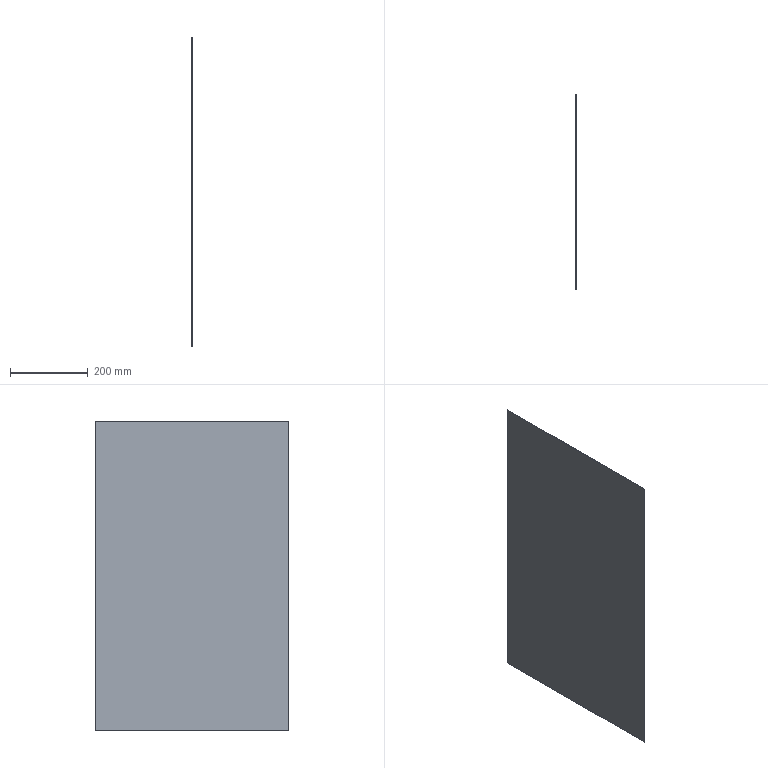Part | SolidWorks | features FlatPattern 1, SMBaseFlange 1, SheetMetal 1 | 1 solid | 6 faces | box 1.2 x 498.8 x 797.6 mm | volume 477411 mm3 | plane 6
STEP:
#1=CARTESIAN_POINT('',(165.125,151.045,-398.8));
#2=VERTEX_POINT('',#1);
#3=CARTESIAN_POINT('',(165.125,649.845,-398.8));
#4=VERTEX_POINT('',#3);
#5=CARTESIAN_POINT('',(165.125,151.045,-398.8));
#6=DIRECTION('',(0.,1.,0.));
#7=VECTOR('',#6,1000.);
#8=LINE('',#5,#7);
#9=EDGE_CURVE('',#2,#4,#8,.T.);
#10=ORIENTED_EDGE('',*,*,#9,.T.);
#11=CARTESIAN_POINT('',(165.125,649.845,398.8));
#12=VERTEX_POINT('',#11);
#13=CARTESIAN_POINT('',(165.125,649.845,398.8));
#14=DIRECTION('',(0.,0.,-1.));
#15=VECTOR('',#14,1000.);
#16=LINE('',#13,#15);
#17=EDGE_CURVE('',#12,#4,#16,.T.);
#18=ORIENTED_EDGE('',*,*,#17,.F.);
#19=CARTESIAN_POINT('',(165.125,151.045,398.8));
#20=VERTEX_POINT('',#19);
#21=CARTESIAN_POINT('',(165.125,151.045,398.8));
#22=DIRECTION('',(0.,1.,0.));
#23=VECTOR('',#22,1000.);
#24=LINE('',#21,#23);
#25=EDGE_CURVE('',#20,#12,#24,.T.);
#26=ORIENTED_EDGE('',*,*,#25,.F.);
#27=CARTESIAN_POINT('',(165.125,151.045,398.8));
#28=DIRECTION('',(0.,0.,-1.));
#29=VECTOR('',#28,1000.);
#30=LINE('',#27,#29);
#31=EDGE_CURVE('',#20,#2,#30,.T.);
#32=ORIENTED_EDGE('',*,*,#31,.T.);
#33=EDGE_LOOP('',(#10,#18,#26,#32));
#34=FACE_OUTER_BOUND('',#33,.T.);
#35=CARTESIAN_POINT('',(165.125,151.045,398.8));
#36=DIRECTION('',(-1.,0.,0.));
#37=DIRECTION('',(0.,0.,1.));
#38=AXIS2_PLACEMENT_3D('',#35,#36,#37);
#39=PLANE('',#38);
#40=ADVANCED_FACE('',(#34),#39,.F.);
#41=CARTESIAN_POINT('',(163.925,649.845,-398.8));
#42=VERTEX_POINT('',#41);
#43=CARTESIAN_POINT('',(163.925,649.845,-398.8));
#44=DIRECTION('',(1.,0.,0.));
#45=VECTOR('',#44,1000.);
#46=LINE('',#43,#45);
#47=EDGE_CURVE('',#42,#4,#46,.T.);
#48=ORIENTED_EDGE('',*,*,#47,.F.);
#49=CARTESIAN_POINT('',(163.925,649.845,398.8));
#50=VERTEX_POINT('',#49);
#51=CARTESIAN_POINT('',(163.925,649.845,398.8));
#52=DIRECTION('',(0.,0.,-1.));
#53=VECTOR('',#52,1000.);
#54=LINE('',#51,#53);
#55=EDGE_CURVE('',#50,#42,#54,.T.);
#56=ORIENTED_EDGE('',*,*,#55,.F.);
#57=CARTESIAN_POINT('',(163.925,649.845,398.8));
#58=DIRECTION('',(1.,0.,0.));
#59=VECTOR('',#58,1000.);
#60=LINE('',#57,#59);
#61=EDGE_CURVE('',#50,#12,#60,.T.);
#62=ORIENTED_EDGE('',*,*,#61,.T.);
#63=ORIENTED_EDGE('',*,*,#17,.T.);
#64=EDGE_LOOP('',(#48,#56,#62,#63));
#65=FACE_OUTER_BOUND('',#64,.T.);
#66=CARTESIAN_POINT('',(163.925,649.845,398.8));
#67=DIRECTION('',(0.,1.,0.));
#68=DIRECTION('',(0.,0.,1.));
#69=AXIS2_PLACEMENT_3D('',#66,#67,#68);
#70=PLANE('',#69);
#71=ADVANCED_FACE('',(#65),#70,.T.);
#72=CARTESIAN_POINT('',(163.925,151.045,-398.8));
#73=VERTEX_POINT('',#72);
#74=CARTESIAN_POINT('',(163.925,151.045,-398.8));
#75=DIRECTION('',(0.,1.,0.));
#76=VECTOR('',#75,1000.);
#77=LINE('',#74,#76);
#78=EDGE_CURVE('',#73,#42,#77,.T.);
#79=ORIENTED_EDGE('',*,*,#78,.F.);
#80=CARTESIAN_POINT('',(163.925,151.045,398.8));
#81=VERTEX_POINT('',#80);
#82=CARTESIAN_POINT('',(163.925,151.045,398.8));
#83=DIRECTION('',(0.,0.,-1.));
#84=VECTOR('',#83,1000.);
#85=LINE('',#82,#84);
#86=EDGE_CURVE('',#81,#73,#85,.T.);
#87=ORIENTED_EDGE('',*,*,#86,.F.);
#88=CARTESIAN_POINT('',(163.925,151.045,398.8));
#89=DIRECTION('',(0.,1.,0.));
#90=VECTOR('',#89,1000.);
#91=LINE('',#88,#90);
#92=EDGE_CURVE('',#81,#50,#91,.T.);
#93=ORIENTED_EDGE('',*,*,#92,.T.);
#94=ORIENTED_EDGE('',*,*,#55,.T.);
#95=EDGE_LOOP('',(#79,#87,#93,#94));
#96=FACE_OUTER_BOUND('',#95,.T.);
#97=CARTESIAN_POINT('',(163.925,151.045,398.8));
#98=DIRECTION('',(-1.,0.,0.));
#99=DIRECTION('',(0.,0.,1.));
#100=AXIS2_PLACEMENT_3D('',#97,#98,#99);
#101=PLANE('',#100);
#102=ADVANCED_FACE('',(#96),#101,.T.);
#103=CARTESIAN_POINT('',(165.125,151.045,-398.8));
#104=DIRECTION('',(-1.,0.,0.));
#105=VECTOR('',#104,1000.);
#106=LINE('',#103,#105);
#107=EDGE_CURVE('',#2,#73,#106,.T.);
#108=ORIENTED_EDGE('',*,*,#107,.F.);
#109=ORIENTED_EDGE('',*,*,#31,.F.);
#110=CARTESIAN_POINT('',(165.125,151.045,398.8));
#111=DIRECTION('',(-1.,0.,0.));
#112=VECTOR('',#111,1000.);
#113=LINE('',#110,#112);
#114=EDGE_CURVE('',#20,#81,#113,.T.);
#115=ORIENTED_EDGE('',*,*,#114,.T.);
#116=ORIENTED_EDGE('',*,*,#86,.T.);
#117=EDGE_LOOP('',(#108,#109,#115,#116));
#118=FACE_OUTER_BOUND('',#117,.T.);
#119=CARTESIAN_POINT('',(165.125,151.045,398.8));
#120=DIRECTION('',(0.,-1.,0.));
#121=DIRECTION('',(0.,0.,-1.));
#122=AXIS2_PLACEMENT_3D('',#119,#120,#121);
#123=PLANE('',#122);
#124=ADVANCED_FACE('',(#118),#123,.T.);
#125=ORIENTED_EDGE('',*,*,#25,.T.);
#126=ORIENTED_EDGE('',*,*,#61,.F.);
#127=ORIENTED_EDGE('',*,*,#92,.F.);
#128=ORIENTED_EDGE('',*,*,#114,.F.);
#129=EDGE_LOOP('',(#125,#126,#127,#128));
#130=FACE_OUTER_BOUND('',#129,.T.);
#131=CARTESIAN_POINT('',(0.,0.,398.8));
#132=DIRECTION('',(0.,0.,-1.));
#133=DIRECTION('',(-1.,0.,0.));
#134=AXIS2_PLACEMENT_3D('',#131,#132,#133);
#135=PLANE('',#134);
#136=ADVANCED_FACE('',(#130),#135,.F.);
#137=ORIENTED_EDGE('',*,*,#9,.F.);
#138=ORIENTED_EDGE('',*,*,#107,.T.);
#139=ORIENTED_EDGE('',*,*,#78,.T.);
#140=ORIENTED_EDGE('',*,*,#47,.T.);
#141=EDGE_LOOP('',(#137,#138,#139,#140));
#142=FACE_OUTER_BOUND('',#141,.T.);
#143=CARTESIAN_POINT('',(0.,0.,-398.8));
#144=DIRECTION('',(0.,0.,-1.));
#145=DIRECTION('',(-1.,0.,0.));
#146=AXIS2_PLACEMENT_3D('',#143,#144,#145);
#147=PLANE('',#146);
#148=ADVANCED_FACE('',(#142),#147,.T.);
#149=CLOSED_SHELL('',(#40,#71,#102,#124,#136,#148));
#150=MANIFOLD_SOLID_BREP('',#149);
#151=CARTESIAN_POINT('',(0.,0.,0.));
#152=DIRECTION('',(0.,0.,1.));
#153=DIRECTION('',(1.,0.,0.));
#154=AXIS2_PLACEMENT_3D('',#151,#152,#153);
#155=(LENGTH_UNIT()NAMED_UNIT(*)SI_UNIT(.MILLI.,.METRE.));
#156=UNCERTAINTY_MEASURE_WITH_UNIT(LENGTH_MEASURE(0.00001),#155,'','');
#157=(NAMED_UNIT(*)PLANE_ANGLE_UNIT()SI_UNIT($,.RADIAN.));
#158=(NAMED_UNIT(*)SI_UNIT($,.STERADIAN.)SOLID_ANGLE_UNIT());
#159=(GEOMETRIC_REPRESENTATION_CONTEXT(3)GLOBAL_UNCERTAINTY_ASSIGNED_CONTEXT((#156))GLOBAL_UNIT_ASSIGNED_CONTEXT((#155,#157,#158))REPRESENTATION_CONTEXT('',''));
#160=ADVANCED_BREP_SHAPE_REPRESENTATION('',(#150,#154),#159);